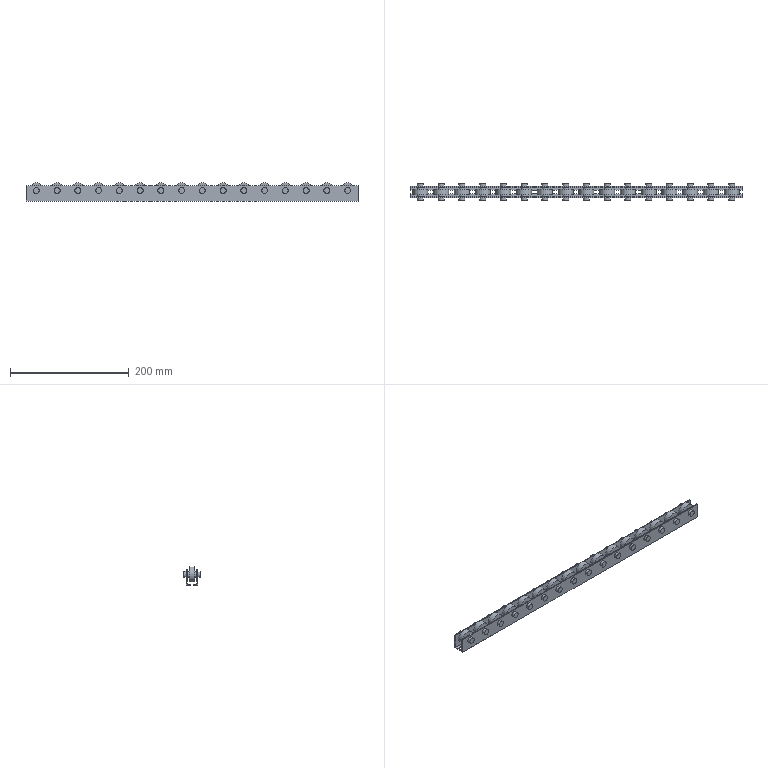Part | NX | features solid 2 | 1 solid | 160 faces | box 560 x 29 x 30.5 mm | volume 150346 mm3 | cylinder 80 | plane 80 | commonest cylinder face diameters 10 x64 25.4 x16